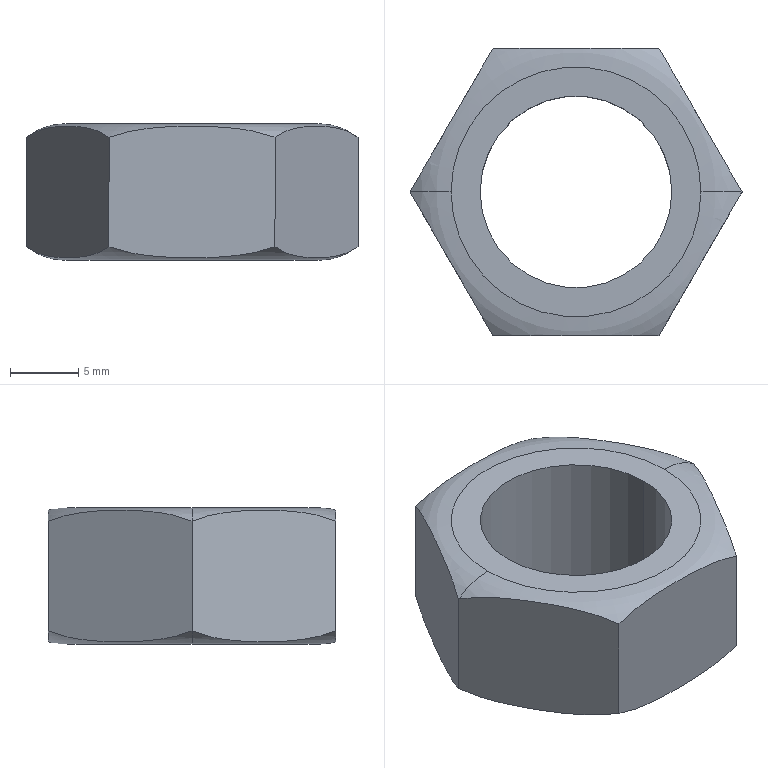Part | SolidWorks | features Extrusion 1, ICE 1, RevCut 1 | 1 solid | 14 faces | box 24.249 x 21 x 10 mm | volume 2242 mm3 | plane 8 | torus 4 | cylinder 2 | commonest cylinder face diameters 14 x2
STEP:
#1=CARTESIAN_POINT('',(7.,0.,10.));
#2=VERTEX_POINT('',#1);
#3=CARTESIAN_POINT('',(-7.,0.,10.));
#4=VERTEX_POINT('',#3);
#5=CARTESIAN_POINT('',(0.,0.,10.));
#6=DIRECTION('',(0.,0.,-1.));
#7=DIRECTION('',(-1.,0.,0.));
#8=AXIS2_PLACEMENT_3D('',#5,#6,#7);
#9=CIRCLE('',#8,7.);
#10=EDGE_CURVE('',#2,#4,#9,.T.);
#11=ORIENTED_EDGE('',*,*,#10,.F.);
#12=CARTESIAN_POINT('',(7.,0.,0.));
#13=VERTEX_POINT('',#12);
#14=CARTESIAN_POINT('',(7.,0.,10.));
#15=DIRECTION('',(0.,0.,-1.));
#16=VECTOR('',#15,1000.);
#17=LINE('',#14,#16);
#18=EDGE_CURVE('',#2,#13,#17,.T.);
#19=ORIENTED_EDGE('',*,*,#18,.T.);
#20=CARTESIAN_POINT('',(-7.,0.,0.));
#21=VERTEX_POINT('',#20);
#22=CARTESIAN_POINT('',(0.,0.,0.));
#23=DIRECTION('',(0.,0.,-1.));
#24=DIRECTION('',(-1.,0.,0.));
#25=AXIS2_PLACEMENT_3D('',#22,#23,#24);
#26=CIRCLE('',#25,7.);
#27=EDGE_CURVE('',#13,#21,#26,.T.);
#28=ORIENTED_EDGE('',*,*,#27,.T.);
#29=CARTESIAN_POINT('',(-7.,0.,10.));
#30=DIRECTION('',(0.,0.,-1.));
#31=VECTOR('',#30,1000.);
#32=LINE('',#29,#31);
#33=EDGE_CURVE('',#4,#21,#32,.T.);
#34=ORIENTED_EDGE('',*,*,#33,.F.);
#35=EDGE_LOOP('',(#11,#19,#28,#34));
#36=FACE_OUTER_BOUND('',#35,.T.);
#37=CARTESIAN_POINT('',(0.,0.,10.));
#38=DIRECTION('',(0.,0.,-1.));
#39=DIRECTION('',(-1.,0.,0.));
#40=AXIS2_PLACEMENT_3D('',#37,#38,#39);
#41=CYLINDRICAL_SURFACE('',#40,7.);
#42=ADVANCED_FACE('',(#36),#41,.F.);
#43=CARTESIAN_POINT('',(-9.124,0.,10.));
#44=VERTEX_POINT('',#43);
#45=CARTESIAN_POINT('',(9.124,0.,10.));
#46=VERTEX_POINT('',#45);
#47=CARTESIAN_POINT('',(0.,0.,10.));
#48=DIRECTION('',(0.,0.,-1.));
#49=DIRECTION('',(-1.,0.,0.));
#50=AXIS2_PLACEMENT_3D('',#47,#48,#49);
#51=CIRCLE('',#50,9.124);
#52=EDGE_CURVE('',#44,#46,#51,.T.);
#53=ORIENTED_EDGE('',*,*,#52,.T.);
#54=CARTESIAN_POINT('',(12.124,0.,9.));
#55=VERTEX_POINT('',#54);
#56=CARTESIAN_POINT('',(9.124,0.,5.));
#57=DIRECTION('',(0.,1.,0.));
#58=DIRECTION('',(-1.,0.,0.));
#59=AXIS2_PLACEMENT_3D('',#56,#57,#58);
#60=CIRCLE('',#59,5.);
#61=EDGE_CURVE('',#46,#55,#60,.T.);
#62=ORIENTED_EDGE('',*,*,#61,.T.);
#63=CARTESIAN_POINT('',(6.062,10.5,9.));
#64=VERTEX_POINT('',#63);
#65=CARTESIAN_POINT('',(6.062,10.5,9.));
#66=CARTESIAN_POINT('',(6.304,10.08,9.182));
#67=CARTESIAN_POINT('',(6.551,9.653,9.317));
#68=CARTESIAN_POINT('',(7.05,8.789,9.528));
#69=CARTESIAN_POINT('',(7.303,8.351,9.603));
#70=CARTESIAN_POINT('',(7.811,7.47,9.714));
#71=CARTESIAN_POINT('',(8.068,7.026,9.75));
#72=CARTESIAN_POINT('',(8.58,6.139,9.797));
#73=CARTESIAN_POINT('',(8.835,5.696,9.807));
#74=CARTESIAN_POINT('',(9.346,4.812,9.807));
#75=CARTESIAN_POINT('',(9.602,4.37,9.797));
#76=CARTESIAN_POINT('',(10.112,3.486,9.751));
#77=CARTESIAN_POINT('',(10.366,3.045,9.716));
#78=CARTESIAN_POINT('',(10.875,2.164,9.605));
#79=CARTESIAN_POINT('',(11.13,1.722,9.53));
#80=CARTESIAN_POINT('',(11.634,0.8487,9.318));
#81=CARTESIAN_POINT('',(11.882,0.419,9.181));
#82=CARTESIAN_POINT('',(12.124,0.,9.));
#83=B_SPLINE_CURVE_WITH_KNOTS('',3,(#65,#66,#67,#68,#69,#70,#71,#72,#73,#74,#75,#76,#77,#78,#79,#80,#81,#82),.UNSPECIFIED.,.F.,.F.,(4,2,2,2,2,2,2,2,4),(0.000000243,0.00153,0.003061,0.004591,0.006121,0.007651,0.009181,0.01071,0.01224),.UNSPECIFIED.);
#84=EDGE_CURVE('',#64,#55,#83,.T.);
#85=ORIENTED_EDGE('',*,*,#84,.F.);
#86=CARTESIAN_POINT('',(-6.062,10.5,9.));
#87=VERTEX_POINT('',#86);
#88=CARTESIAN_POINT('',(-6.062,10.5,9.));
#89=CARTESIAN_POINT('',(-5.582,10.5,9.18));
#90=CARTESIAN_POINT('',(-5.091,10.5,9.315));
#91=CARTESIAN_POINT('',(-4.093,10.5,9.526));
#92=CARTESIAN_POINT('',(-3.587,10.5,9.602));
#93=CARTESIAN_POINT('',(-2.567,10.5,9.714));
#94=CARTESIAN_POINT('',(-2.056,10.5,9.75));
#95=CARTESIAN_POINT('',(-1.033,10.5,9.796));
#96=CARTESIAN_POINT('',(-0.5206,10.5,9.807));
#97=CARTESIAN_POINT('',(0.5051,10.5,9.807));
#98=CARTESIAN_POINT('',(1.018,10.5,9.797));
#99=CARTESIAN_POINT('',(2.041,10.5,9.751));
#100=CARTESIAN_POINT('',(2.551,10.5,9.715));
#101=CARTESIAN_POINT('',(3.568,10.5,9.605));
#102=CARTESIAN_POINT('',(4.074,10.5,9.53));
#103=CARTESIAN_POINT('',(5.081,10.5,9.318));
#104=CARTESIAN_POINT('',(5.581,10.5,9.181));
#105=CARTESIAN_POINT('',(6.062,10.5,9.));
#106=B_SPLINE_CURVE_WITH_KNOTS('',3,(#88,#89,#90,#91,#92,#93,#94,#95,#96,#97,#98,#99,#100,#101,#102,#103,#104,#105),.UNSPECIFIED.,.F.,.F.,(4,2,2,2,2,2,2,2,4),(0.04063,0.04216,0.0437,0.04523,0.04676,0.0483,0.04983,0.05136,0.0529),.UNSPECIFIED.);
#107=EDGE_CURVE('',#87,#64,#106,.T.);
#108=ORIENTED_EDGE('',*,*,#107,.F.);
#109=CARTESIAN_POINT('',(-12.124,0.,9.));
#110=VERTEX_POINT('',#109);
#111=CARTESIAN_POINT('',(-12.124,0.,9.));
#112=CARTESIAN_POINT('',(-11.882,0.4195,9.182));
#113=CARTESIAN_POINT('',(-11.635,0.8468,9.317));
#114=CARTESIAN_POINT('',(-11.136,1.711,9.528));
#115=CARTESIAN_POINT('',(-10.884,2.149,9.603));
#116=CARTESIAN_POINT('',(-10.375,3.03,9.714));
#117=CARTESIAN_POINT('',(-10.118,3.474,9.75));
#118=CARTESIAN_POINT('',(-9.607,4.361,9.797));
#119=CARTESIAN_POINT('',(-9.351,4.804,9.807));
#120=CARTESIAN_POINT('',(-8.84,5.688,9.807));
#121=CARTESIAN_POINT('',(-8.585,6.13,9.797));
#122=CARTESIAN_POINT('',(-8.075,7.014,9.751));
#123=CARTESIAN_POINT('',(-7.82,7.455,9.716));
#124=CARTESIAN_POINT('',(-7.311,8.336,9.605));
#125=CARTESIAN_POINT('',(-7.056,8.778,9.53));
#126=CARTESIAN_POINT('',(-6.552,9.651,9.318));
#127=CARTESIAN_POINT('',(-6.304,10.081,9.181));
#128=CARTESIAN_POINT('',(-6.062,10.5,9.));
#129=B_SPLINE_CURVE_WITH_KNOTS('',3,(#111,#112,#113,#114,#115,#116,#117,#118,#119,#120,#121,#122,#123,#124,#125,#126,#127,#128),.UNSPECIFIED.,.F.,.F.,(4,2,2,2,2,2,2,2,4),(0.000000243,0.00153,0.003061,0.004591,0.006121,0.007651,0.009181,0.01071,0.01224),.UNSPECIFIED.);
#130=EDGE_CURVE('',#110,#87,#129,.T.);
#131=ORIENTED_EDGE('',*,*,#130,.F.);
#132=CARTESIAN_POINT('',(-9.124,0.,5.));
#133=DIRECTION('',(0.,-1.,0.));
#134=DIRECTION('',(0.,0.,-1.));
#135=AXIS2_PLACEMENT_3D('',#132,#133,#134);
#136=CIRCLE('',#135,5.);
#137=EDGE_CURVE('',#44,#110,#136,.T.);
#138=ORIENTED_EDGE('',*,*,#137,.F.);
#139=EDGE_LOOP('',(#53,#62,#85,#108,#131,#138));
#140=FACE_OUTER_BOUND('',#139,.T.);
#141=CARTESIAN_POINT('',(0.,0.,5.));
#142=DIRECTION('',(0.,0.,-1.));
#143=DIRECTION('',(-1.,0.,0.));
#144=AXIS2_PLACEMENT_3D('',#141,#142,#143);
#145=TOROIDAL_SURFACE('',#144,9.124,5.);
#146=ADVANCED_FACE('',(#140),#145,.T.);
#147=CARTESIAN_POINT('',(12.124,0.,1.));
#148=VERTEX_POINT('',#147);
#149=CARTESIAN_POINT('',(6.062,10.5,1.));
#150=VERTEX_POINT('',#149);
#151=CARTESIAN_POINT('',(12.124,0.,1.));
#152=CARTESIAN_POINT('',(11.882,0.4195,0.8183));
#153=CARTESIAN_POINT('',(11.635,0.8468,0.6831));
#154=CARTESIAN_POINT('',(11.136,1.711,0.4723));
#155=CARTESIAN_POINT('',(10.884,2.149,0.3971));
#156=CARTESIAN_POINT('',(10.375,3.03,0.2857));
#157=CARTESIAN_POINT('',(10.118,3.474,0.2496));
#158=CARTESIAN_POINT('',(9.607,4.361,0.2034));
#159=CARTESIAN_POINT('',(9.351,4.804,0.193));
#160=CARTESIAN_POINT('',(8.84,5.688,0.1929));
#161=CARTESIAN_POINT('',(8.585,6.13,0.2031));
#162=CARTESIAN_POINT('',(8.075,7.014,0.2488));
#163=CARTESIAN_POINT('',(7.82,7.455,0.2843));
#164=CARTESIAN_POINT('',(7.311,8.336,0.3947));
#165=CARTESIAN_POINT('',(7.056,8.778,0.47));
#166=CARTESIAN_POINT('',(6.552,9.651,0.6823));
#167=CARTESIAN_POINT('',(6.304,10.081,0.8186));
#168=CARTESIAN_POINT('',(6.062,10.5,1.));
#169=B_SPLINE_CURVE_WITH_KNOTS('',3,(#151,#152,#153,#154,#155,#156,#157,#158,#159,#160,#161,#162,#163,#164,#165,#166,#167,#168),.UNSPECIFIED.,.F.,.F.,(4,2,2,2,2,2,2,2,4),(0.000000243,0.00153,0.003061,0.004591,0.006121,0.007651,0.009181,0.01071,0.01224),.UNSPECIFIED.);
#170=EDGE_CURVE('',#148,#150,#169,.T.);
#171=ORIENTED_EDGE('',*,*,#170,.F.);
#172=CARTESIAN_POINT('',(9.124,0.,0.));
#173=VERTEX_POINT('',#172);
#174=CARTESIAN_POINT('',(9.124,0.,5.));
#175=DIRECTION('',(0.,1.,0.));
#176=DIRECTION('',(-1.,0.,0.));
#177=AXIS2_PLACEMENT_3D('',#174,#175,#176);
#178=CIRCLE('',#177,5.);
#179=EDGE_CURVE('',#148,#173,#178,.T.);
#180=ORIENTED_EDGE('',*,*,#179,.T.);
#181=CARTESIAN_POINT('',(-9.124,0.,0.));
#182=VERTEX_POINT('',#181);
#183=CARTESIAN_POINT('',(0.,0.,0.));
#184=DIRECTION('',(0.,0.,-1.));
#185=DIRECTION('',(-1.,0.,0.));
#186=AXIS2_PLACEMENT_3D('',#183,#184,#185);
#187=CIRCLE('',#186,9.124);
#188=EDGE_CURVE('',#182,#173,#187,.T.);
#189=ORIENTED_EDGE('',*,*,#188,.F.);
#190=CARTESIAN_POINT('',(-12.124,0.,1.));
#191=VERTEX_POINT('',#190);
#192=CARTESIAN_POINT('',(-9.124,0.,5.));
#193=DIRECTION('',(0.,-1.,0.));
#194=DIRECTION('',(0.,0.,-1.));
#195=AXIS2_PLACEMENT_3D('',#192,#193,#194);
#196=CIRCLE('',#195,5.);
#197=EDGE_CURVE('',#191,#182,#196,.T.);
#198=ORIENTED_EDGE('',*,*,#197,.F.);
#199=CARTESIAN_POINT('',(-6.062,10.5,1.));
#200=VERTEX_POINT('',#199);
#201=CARTESIAN_POINT('',(-6.062,10.5,1.));
#202=CARTESIAN_POINT('',(-6.304,10.08,0.8183));
#203=CARTESIAN_POINT('',(-6.551,9.653,0.6831));
#204=CARTESIAN_POINT('',(-7.05,8.789,0.4723));
#205=CARTESIAN_POINT('',(-7.303,8.351,0.3971));
#206=CARTESIAN_POINT('',(-7.811,7.47,0.2857));
#207=CARTESIAN_POINT('',(-8.068,7.026,0.2496));
#208=CARTESIAN_POINT('',(-8.58,6.139,0.2034));
#209=CARTESIAN_POINT('',(-8.835,5.696,0.193));
#210=CARTESIAN_POINT('',(-9.346,4.812,0.1929));
#211=CARTESIAN_POINT('',(-9.602,4.37,0.2031));
#212=CARTESIAN_POINT('',(-10.112,3.486,0.2488));
#213=CARTESIAN_POINT('',(-10.366,3.045,0.2843));
#214=CARTESIAN_POINT('',(-10.875,2.164,0.3947));
#215=CARTESIAN_POINT('',(-11.13,1.722,0.47));
#216=CARTESIAN_POINT('',(-11.634,0.8487,0.6823));
#217=CARTESIAN_POINT('',(-11.882,0.419,0.8186));
#218=CARTESIAN_POINT('',(-12.124,0.,1.));
#219=B_SPLINE_CURVE_WITH_KNOTS('',3,(#201,#202,#203,#204,#205,#206,#207,#208,#209,#210,#211,#212,#213,#214,#215,#216,#217,#218),.UNSPECIFIED.,.F.,.F.,(4,2,2,2,2,2,2,2,4),(0.000000243,0.00153,0.003061,0.004591,0.006121,0.007651,0.009181,0.01071,0.01224),.UNSPECIFIED.);
#220=EDGE_CURVE('',#200,#191,#219,.T.);
#221=ORIENTED_EDGE('',*,*,#220,.F.);
#222=CARTESIAN_POINT('',(6.062,10.5,1.));
#223=CARTESIAN_POINT('',(5.582,10.5,0.8199));
#224=CARTESIAN_POINT('',(5.091,10.5,0.6847));
#225=CARTESIAN_POINT('',(4.093,10.5,0.4736));
#226=CARTESIAN_POINT('',(3.587,10.5,0.3979));
#227=CARTESIAN_POINT('',(2.567,10.5,0.286));
#228=CARTESIAN_POINT('',(2.056,10.5,0.25));
#229=CARTESIAN_POINT('',(1.033,10.5,0.2035));
#230=CARTESIAN_POINT('',(0.5206,10.5,0.1931));
#231=CARTESIAN_POINT('',(-0.5051,10.5,0.1929));
#232=CARTESIAN_POINT('',(-1.018,10.5,0.2031));
#233=CARTESIAN_POINT('',(-2.041,10.5,0.249));
#234=CARTESIAN_POINT('',(-2.551,10.5,0.2847));
#235=CARTESIAN_POINT('',(-3.568,10.5,0.3953));
#236=CARTESIAN_POINT('',(-4.074,10.5,0.4702));
#237=CARTESIAN_POINT('',(-5.081,10.5,0.6821));
#238=CARTESIAN_POINT('',(-5.581,10.5,0.8195));
#239=CARTESIAN_POINT('',(-6.062,10.5,1.));
#240=B_SPLINE_CURVE_WITH_KNOTS('',3,(#222,#223,#224,#225,#226,#227,#228,#229,#230,#231,#232,#233,#234,#235,#236,#237,#238,#239),.UNSPECIFIED.,.F.,.F.,(4,2,2,2,2,2,2,2,4),(0.04063,0.04216,0.0437,0.04523,0.04676,0.0483,0.04983,0.05136,0.0529),.UNSPECIFIED.);
#241=EDGE_CURVE('',#150,#200,#240,.T.);
#242=ORIENTED_EDGE('',*,*,#241,.F.);
#243=EDGE_LOOP('',(#171,#180,#189,#198,#221,#242));
#244=FACE_OUTER_BOUND('',#243,.T.);
#245=CARTESIAN_POINT('',(0.,0.,5.));
#246=DIRECTION('',(0.,0.,-1.));
#247=DIRECTION('',(-1.,0.,0.));
#248=AXIS2_PLACEMENT_3D('',#245,#246,#247);
#249=TOROIDAL_SURFACE('',#248,9.124,5.);
#250=ADVANCED_FACE('',(#244),#249,.T.);
#251=CARTESIAN_POINT('',(12.124,0.,10.));
#252=DIRECTION('',(0.,0.,-1.));
#253=VECTOR('',#252,1000.);
#254=LINE('',#251,#253);
#255=EDGE_CURVE('',#55,#148,#254,.T.);
#256=ORIENTED_EDGE('',*,*,#255,.F.);
#257=CARTESIAN_POINT('',(6.062,-10.5,9.));
#258=VERTEX_POINT('',#257);
#259=CARTESIAN_POINT('',(12.124,0.,9.));
#260=CARTESIAN_POINT('',(11.882,-0.4195,9.182));
#261=CARTESIAN_POINT('',(11.635,-0.8468,9.317));
#262=CARTESIAN_POINT('',(11.136,-1.711,9.528));
#263=CARTESIAN_POINT('',(10.884,-2.149,9.603));
#264=CARTESIAN_POINT('',(10.375,-3.03,9.714));
#265=CARTESIAN_POINT('',(10.118,-3.474,9.75));
#266=CARTESIAN_POINT('',(9.607,-4.361,9.797));
#267=CARTESIAN_POINT('',(9.351,-4.804,9.807));
#268=CARTESIAN_POINT('',(8.84,-5.688,9.807));
#269=CARTESIAN_POINT('',(8.585,-6.13,9.797));
#270=CARTESIAN_POINT('',(8.075,-7.014,9.751));
#271=CARTESIAN_POINT('',(7.82,-7.455,9.716));
#272=CARTESIAN_POINT('',(7.311,-8.336,9.605));
#273=CARTESIAN_POINT('',(7.056,-8.778,9.53));
#274=CARTESIAN_POINT('',(6.552,-9.651,9.318));
#275=CARTESIAN_POINT('',(6.304,-10.081,9.181));
#276=CARTESIAN_POINT('',(6.062,-10.5,9.));
#277=B_SPLINE_CURVE_WITH_KNOTS('',3,(#259,#260,#261,#262,#263,#264,#265,#266,#267,#268,#269,#270,#271,#272,#273,#274,#275,#276),.UNSPECIFIED.,.F.,.F.,(4,2,2,2,2,2,2,2,4),(0.000000243,0.00153,0.003061,0.004591,0.006121,0.007651,0.009181,0.01071,0.01224),.UNSPECIFIED.);
#278=EDGE_CURVE('',#55,#258,#277,.T.);
#279=ORIENTED_EDGE('',*,*,#278,.T.);
#280=CARTESIAN_POINT('',(6.062,-10.5,1.));
#281=VERTEX_POINT('',#280);
#282=CARTESIAN_POINT('',(6.062,-10.5,10.));
#283=DIRECTION('',(0.,0.,-1.));
#284=VECTOR('',#283,1000.);
#285=LINE('',#282,#284);
#286=EDGE_CURVE('',#258,#281,#285,.T.);
#287=ORIENTED_EDGE('',*,*,#286,.T.);
#288=CARTESIAN_POINT('',(6.062,-10.5,1.));
#289=CARTESIAN_POINT('',(6.304,-10.08,0.8183));
#290=CARTESIAN_POINT('',(6.551,-9.653,0.6831));
#291=CARTESIAN_POINT('',(7.05,-8.789,0.4723));
#292=CARTESIAN_POINT('',(7.303,-8.351,0.3971));
#293=CARTESIAN_POINT('',(7.811,-7.47,0.2857));
#294=CARTESIAN_POINT('',(8.068,-7.026,0.2496));
#295=CARTESIAN_POINT('',(8.58,-6.139,0.2034));
#296=CARTESIAN_POINT('',(8.835,-5.696,0.193));
#297=CARTESIAN_POINT('',(9.346,-4.812,0.1929));
#298=CARTESIAN_POINT('',(9.602,-4.37,0.2031));
#299=CARTESIAN_POINT('',(10.112,-3.486,0.2488));
#300=CARTESIAN_POINT('',(10.366,-3.045,0.2843));
#301=CARTESIAN_POINT('',(10.875,-2.164,0.3947));
#302=CARTESIAN_POINT('',(11.13,-1.722,0.47));
#303=CARTESIAN_POINT('',(11.634,-0.8487,0.6823));
#304=CARTESIAN_POINT('',(11.882,-0.419,0.8186));
#305=CARTESIAN_POINT('',(12.124,0.,1.));
#306=B_SPLINE_CURVE_WITH_KNOTS('',3,(#288,#289,#290,#291,#292,#293,#294,#295,#296,#297,#298,#299,#300,#301,#302,#303,#304,#305),.UNSPECIFIED.,.F.,.F.,(4,2,2,2,2,2,2,2,4),(0.000000243,0.00153,0.003061,0.004591,0.006121,0.007651,0.009181,0.01071,0.01224),.UNSPECIFIED.);
#307=EDGE_CURVE('',#281,#148,#306,.T.);
#308=ORIENTED_EDGE('',*,*,#307,.T.);
#309=EDGE_LOOP('',(#256,#279,#287,#308));
#310=FACE_OUTER_BOUND('',#309,.T.);
#311=CARTESIAN_POINT('',(6.062,-10.5,10.));
#312=DIRECTION('',(-0.866,0.5,0.));
#313=DIRECTION('',(-0.5,-0.866,0.));
#314=AXIS2_PLACEMENT_3D('',#311,#312,#313);
#315=PLANE('',#314);
#316=ADVANCED_FACE('',(#310),#315,.F.);
#317=CARTESIAN_POINT('',(6.062,10.5,10.));
#318=DIRECTION('',(0.,0.,-1.));
#319=VECTOR('',#318,1000.);
#320=LINE('',#317,#319);
#321=EDGE_CURVE('',#64,#150,#320,.T.);
#322=ORIENTED_EDGE('',*,*,#321,.F.);
#323=ORIENTED_EDGE('',*,*,#84,.T.);
#324=ORIENTED_EDGE('',*,*,#255,.T.);
#325=ORIENTED_EDGE('',*,*,#170,.T.);
#326=EDGE_LOOP('',(#322,#323,#324,#325));
#327=FACE_OUTER_BOUND('',#326,.T.);
#328=CARTESIAN_POINT('',(12.124,0.,10.));
#329=DIRECTION('',(-0.866,-0.5,0.));
#330=DIRECTION('',(0.5,-0.866,0.));
#331=AXIS2_PLACEMENT_3D('',#328,#329,#330);
#332=PLANE('',#331);
#333=ADVANCED_FACE('',(#327),#332,.F.);
#334=CARTESIAN_POINT('',(-6.062,10.5,10.));
#335=DIRECTION('',(0.,0.,-1.));
#336=VECTOR('',#335,1000.);
#337=LINE('',#334,#336);
#338=EDGE_CURVE('',#87,#200,#337,.T.);
#339=ORIENTED_EDGE('',*,*,#338,.F.);
#340=ORIENTED_EDGE('',*,*,#107,.T.);
#341=ORIENTED_EDGE('',*,*,#321,.T.);
#342=ORIENTED_EDGE('',*,*,#241,.T.);
#343=EDGE_LOOP('',(#339,#340,#341,#342));
#344=FACE_OUTER_BOUND('',#343,.T.);
#345=CARTESIAN_POINT('',(6.062,10.5,10.));
#346=DIRECTION('',(0.,-1.,0.));
#347=DIRECTION('',(0.,0.,-1.));
#348=AXIS2_PLACEMENT_3D('',#345,#346,#347);
#349=PLANE('',#348);
#350=ADVANCED_FACE('',(#344),#349,.F.);
#351=CARTESIAN_POINT('',(-12.124,0.,10.));
#352=DIRECTION('',(0.,0.,-1.));
#353=VECTOR('',#352,1000.);
#354=LINE('',#351,#353);
#355=EDGE_CURVE('',#110,#191,#354,.T.);
#356=ORIENTED_EDGE('',*,*,#355,.F.);
#357=ORIENTED_EDGE('',*,*,#130,.T.);
#358=ORIENTED_EDGE('',*,*,#338,.T.);
#359=ORIENTED_EDGE('',*,*,#220,.T.);
#360=EDGE_LOOP('',(#356,#357,#358,#359));
#361=FACE_OUTER_BOUND('',#360,.T.);
#362=CARTESIAN_POINT('',(-6.062,10.5,10.));
#363=DIRECTION('',(0.866,-0.5,0.));
#364=DIRECTION('',(0.5,0.866,0.));
#365=AXIS2_PLACEMENT_3D('',#362,#363,#364);
#366=PLANE('',#365);
#367=ADVANCED_FACE('',(#361),#366,.F.);
#368=CARTESIAN_POINT('',(-6.062,-10.5,9.));
#369=VERTEX_POINT('',#368);
#370=CARTESIAN_POINT('',(-6.062,-10.5,1.));
#371=VERTEX_POINT('',#370);
#372=CARTESIAN_POINT('',(-6.062,-10.5,10.));
#373=DIRECTION('',(0.,0.,-1.));
#374=VECTOR('',#373,1000.);
#375=LINE('',#372,#374);
#376=EDGE_CURVE('',#369,#371,#375,.T.);
#377=ORIENTED_EDGE('',*,*,#376,.F.);
#378=CARTESIAN_POINT('',(-6.062,-10.5,9.));
#379=CARTESIAN_POINT('',(-6.304,-10.08,9.182));
#380=CARTESIAN_POINT('',(-6.551,-9.653,9.317));
#381=CARTESIAN_POINT('',(-7.05,-8.789,9.528));
#382=CARTESIAN_POINT('',(-7.303,-8.351,9.603));
#383=CARTESIAN_POINT('',(-7.811,-7.47,9.714));
#384=CARTESIAN_POINT('',(-8.068,-7.026,9.75));
#385=CARTESIAN_POINT('',(-8.58,-6.139,9.797));
#386=CARTESIAN_POINT('',(-8.835,-5.696,9.807));
#387=CARTESIAN_POINT('',(-9.346,-4.812,9.807));
#388=CARTESIAN_POINT('',(-9.602,-4.37,9.797));
#389=CARTESIAN_POINT('',(-10.112,-3.486,9.751));
#390=CARTESIAN_POINT('',(-10.366,-3.045,9.716));
#391=CARTESIAN_POINT('',(-10.875,-2.164,9.605));
#392=CARTESIAN_POINT('',(-11.13,-1.722,9.53));
#393=CARTESIAN_POINT('',(-11.634,-0.8487,9.318));
#394=CARTESIAN_POINT('',(-11.882,-0.419,9.181));
#395=CARTESIAN_POINT('',(-12.124,0.,9.));
#396=B_SPLINE_CURVE_WITH_KNOTS('',3,(#378,#379,#380,#381,#382,#383,#384,#385,#386,#387,#388,#389,#390,#391,#392,#393,#394,#395),.UNSPECIFIED.,.F.,.F.,(4,2,2,2,2,2,2,2,4),(0.000000243,0.00153,0.003061,0.004591,0.006121,0.007651,0.009181,0.01071,0.01224),.UNSPECIFIED.);
#397=EDGE_CURVE('',#369,#110,#396,.T.);
#398=ORIENTED_EDGE('',*,*,#397,.T.);
#399=ORIENTED_EDGE('',*,*,#355,.T.);
#400=CARTESIAN_POINT('',(-12.124,0.,1.));
#401=CARTESIAN_POINT('',(-11.882,-0.4195,0.8183));
#402=CARTESIAN_POINT('',(-11.635,-0.8468,0.6831));
#403=CARTESIAN_POINT('',(-11.136,-1.711,0.4723));
#404=CARTESIAN_POINT('',(-10.884,-2.149,0.3971));
#405=CARTESIAN_POINT('',(-10.375,-3.03,0.2857));
#406=CARTESIAN_POINT('',(-10.118,-3.474,0.2496));
#407=CARTESIAN_POINT('',(-9.607,-4.361,0.2034));
#408=CARTESIAN_POINT('',(-9.351,-4.804,0.193));
#409=CARTESIAN_POINT('',(-8.84,-5.688,0.1929));
#410=CARTESIAN_POINT('',(-8.585,-6.13,0.2031));
#411=CARTESIAN_POINT('',(-8.075,-7.014,0.2488));
#412=CARTESIAN_POINT('',(-7.82,-7.455,0.2843));
#413=CARTESIAN_POINT('',(-7.311,-8.336,0.3947));
#414=CARTESIAN_POINT('',(-7.056,-8.778,0.47));
#415=CARTESIAN_POINT('',(-6.552,-9.651,0.6823));
#416=CARTESIAN_POINT('',(-6.304,-10.081,0.8186));
#417=CARTESIAN_POINT('',(-6.062,-10.5,1.));
#418=B_SPLINE_CURVE_WITH_KNOTS('',3,(#400,#401,#402,#403,#404,#405,#406,#407,#408,#409,#410,#411,#412,#413,#414,#415,#416,#417),.UNSPECIFIED.,.F.,.F.,(4,2,2,2,2,2,2,2,4),(0.000000243,0.00153,0.003061,0.004591,0.006121,0.007651,0.009181,0.01071,0.01224),.UNSPECIFIED.);
#419=EDGE_CURVE('',#191,#371,#418,.T.);
#420=ORIENTED_EDGE('',*,*,#419,.T.);
#421=EDGE_LOOP('',(#377,#398,#399,#420));
#422=FACE_OUTER_BOUND('',#421,.T.);
#423=CARTESIAN_POINT('',(-12.124,0.,10.));
#424=DIRECTION('',(0.866,0.5,0.));
#425=DIRECTION('',(-0.5,0.866,0.));
#426=AXIS2_PLACEMENT_3D('',#423,#424,#425);
#427=PLANE('',#426);
#428=ADVANCED_FACE('',(#422),#427,.F.);
#429=ORIENTED_EDGE('',*,*,#286,.F.);
#430=CARTESIAN_POINT('',(6.062,-10.5,9.));
#431=CARTESIAN_POINT('',(5.582,-10.5,9.18));
#432=CARTESIAN_POINT('',(5.091,-10.5,9.315));
#433=CARTESIAN_POINT('',(4.093,-10.5,9.526));
#434=CARTESIAN_POINT('',(3.587,-10.5,9.602));
#435=CARTESIAN_POINT('',(2.567,-10.5,9.714));
#436=CARTESIAN_POINT('',(2.056,-10.5,9.75));
#437=CARTESIAN_POINT('',(1.033,-10.5,9.796));
#438=CARTESIAN_POINT('',(0.5206,-10.5,9.807));
#439=CARTESIAN_POINT('',(-0.5051,-10.5,9.807));
#440=CARTESIAN_POINT('',(-1.018,-10.5,9.797));
#441=CARTESIAN_POINT('',(-2.041,-10.5,9.751));
#442=CARTESIAN_POINT('',(-2.551,-10.5,9.715));
#443=CARTESIAN_POINT('',(-3.568,-10.5,9.605));
#444=CARTESIAN_POINT('',(-4.074,-10.5,9.53));
#445=CARTESIAN_POINT('',(-5.081,-10.5,9.318));
#446=CARTESIAN_POINT('',(-5.581,-10.5,9.181));
#447=CARTESIAN_POINT('',(-6.062,-10.5,9.));
#448=B_SPLINE_CURVE_WITH_KNOTS('',3,(#430,#431,#432,#433,#434,#435,#436,#437,#438,#439,#440,#441,#442,#443,#444,#445,#446,#447),.UNSPECIFIED.,.F.,.F.,(4,2,2,2,2,2,2,2,4),(0.04063,0.04216,0.0437,0.04523,0.04676,0.0483,0.04983,0.05136,0.0529),.UNSPECIFIED.);
#449=EDGE_CURVE('',#258,#369,#448,.T.);
#450=ORIENTED_EDGE('',*,*,#449,.T.);
#451=ORIENTED_EDGE('',*,*,#376,.T.);
#452=CARTESIAN_POINT('',(-6.062,-10.5,1.));
#453=CARTESIAN_POINT('',(-5.582,-10.5,0.8199));
#454=CARTESIAN_POINT('',(-5.091,-10.5,0.6847));
#455=CARTESIAN_POINT('',(-4.093,-10.5,0.4736));
#456=CARTESIAN_POINT('',(-3.587,-10.5,0.3979));
#457=CARTESIAN_POINT('',(-2.567,-10.5,0.286));
#458=CARTESIAN_POINT('',(-2.056,-10.5,0.25));
#459=CARTESIAN_POINT('',(-1.033,-10.5,0.2035));
#460=CARTESIAN_POINT('',(-0.5206,-10.5,0.1931));
#461=CARTESIAN_POINT('',(0.5051,-10.5,0.1929));
#462=CARTESIAN_POINT('',(1.018,-10.5,0.2031));
#463=CARTESIAN_POINT('',(2.041,-10.5,0.249));
#464=CARTESIAN_POINT('',(2.551,-10.5,0.2847));
#465=CARTESIAN_POINT('',(3.568,-10.5,0.3953));
#466=CARTESIAN_POINT('',(4.074,-10.5,0.4702));
#467=CARTESIAN_POINT('',(5.081,-10.5,0.6821));
#468=CARTESIAN_POINT('',(5.581,-10.5,0.8195));
#469=CARTESIAN_POINT('',(6.062,-10.5,1.));
#470=B_SPLINE_CURVE_WITH_KNOTS('',3,(#452,#453,#454,#455,#456,#457,#458,#459,#460,#461,#462,#463,#464,#465,#466,#467,#468,#469),.UNSPECIFIED.,.F.,.F.,(4,2,2,2,2,2,2,2,4),(0.04063,0.04216,0.0437,0.04523,0.04676,0.0483,0.04983,0.05136,0.0529),.UNSPECIFIED.);
#471=EDGE_CURVE('',#371,#281,#470,.T.);
#472=ORIENTED_EDGE('',*,*,#471,.T.);
#473=EDGE_LOOP('',(#429,#450,#451,#472));
#474=FACE_OUTER_BOUND('',#473,.T.);
#475=CARTESIAN_POINT('',(-6.062,-10.5,10.));
#476=DIRECTION('',(0.,1.,0.));
#477=DIRECTION('',(0.,0.,1.));
#478=AXIS2_PLACEMENT_3D('',#475,#476,#477);
#479=PLANE('',#478);
#480=ADVANCED_FACE('',(#474),#479,.F.);
#481=ORIENTED_EDGE('',*,*,#179,.F.);
#482=ORIENTED_EDGE('',*,*,#307,.F.);
#483=ORIENTED_EDGE('',*,*,#471,.F.);
#484=ORIENTED_EDGE('',*,*,#419,.F.);
#485=ORIENTED_EDGE('',*,*,#197,.T.);
#486=CARTESIAN_POINT('',(0.,0.,0.));
#487=DIRECTION('',(0.,0.,-1.));
#488=DIRECTION('',(-1.,0.,0.));
#489=AXIS2_PLACEMENT_3D('',#486,#487,#488);
#490=CIRCLE('',#489,9.124);
#491=EDGE_CURVE('',#173,#182,#490,.T.);
#492=ORIENTED_EDGE('',*,*,#491,.F.);
#493=EDGE_LOOP('',(#481,#482,#483,#484,#485,#492));
#494=FACE_OUTER_BOUND('',#493,.T.);
#495=CARTESIAN_POINT('',(0.,0.,5.));
#496=DIRECTION('',(0.,0.,-1.));
#497=DIRECTION('',(-1.,0.,0.));
#498=AXIS2_PLACEMENT_3D('',#495,#496,#497);
#499=TOROIDAL_SURFACE('',#498,9.124,5.);
#500=ADVANCED_FACE('',(#494),#499,.T.);
#501=CARTESIAN_POINT('',(0.,0.,0.));
#502=DIRECTION('',(0.,0.,-1.));
#503=DIRECTION('',(-1.,0.,0.));
#504=AXIS2_PLACEMENT_3D('',#501,#502,#503);
#505=CIRCLE('',#504,7.);
#506=EDGE_CURVE('',#21,#13,#505,.T.);
#507=ORIENTED_EDGE('',*,*,#506,.F.);
#508=ORIENTED_EDGE('',*,*,#27,.F.);
#509=EDGE_LOOP('',(#507,#508));
#510=FACE_BOUND('',#509,.T.);
#511=ORIENTED_EDGE('',*,*,#188,.T.);
#512=ORIENTED_EDGE('',*,*,#491,.T.);
#513=EDGE_LOOP('',(#511,#512));
#514=FACE_OUTER_BOUND('',#513,.T.);
#515=CARTESIAN_POINT('',(0.,0.,0.));
#516=DIRECTION('',(0.,0.,1.));
#517=DIRECTION('',(1.,0.,0.));
#518=AXIS2_PLACEMENT_3D('',#515,#516,#517);
#519=PLANE('',#518);
#520=ADVANCED_FACE('',(#510,#514),#519,.F.);
#521=ORIENTED_EDGE('',*,*,#61,.F.);
#522=CARTESIAN_POINT('',(0.,0.,10.));
#523=DIRECTION('',(0.,0.,-1.));
#524=DIRECTION('',(-1.,0.,0.));
#525=AXIS2_PLACEMENT_3D('',#522,#523,#524);
#526=CIRCLE('',#525,9.124);
#527=EDGE_CURVE('',#46,#44,#526,.T.);
#528=ORIENTED_EDGE('',*,*,#527,.T.);
#529=ORIENTED_EDGE('',*,*,#137,.T.);
#530=ORIENTED_EDGE('',*,*,#397,.F.);
#531=ORIENTED_EDGE('',*,*,#449,.F.);
#532=ORIENTED_EDGE('',*,*,#278,.F.);
#533=EDGE_LOOP('',(#521,#528,#529,#530,#531,#532));
#534=FACE_OUTER_BOUND('',#533,.T.);
#535=CARTESIAN_POINT('',(0.,0.,5.));
#536=DIRECTION('',(0.,0.,-1.));
#537=DIRECTION('',(-1.,0.,0.));
#538=AXIS2_PLACEMENT_3D('',#535,#536,#537);
#539=TOROIDAL_SURFACE('',#538,9.124,5.);
#540=ADVANCED_FACE('',(#534),#539,.T.);
#541=CARTESIAN_POINT('',(0.,0.,10.));
#542=DIRECTION('',(0.,0.,-1.));
#543=DIRECTION('',(-1.,0.,0.));
#544=AXIS2_PLACEMENT_3D('',#541,#542,#543);
#545=CIRCLE('',#544,7.);
#546=EDGE_CURVE('',#4,#2,#545,.T.);
#547=ORIENTED_EDGE('',*,*,#546,.T.);
#548=ORIENTED_EDGE('',*,*,#10,.T.);
#549=EDGE_LOOP('',(#547,#548));
#550=FACE_BOUND('',#549,.T.);
#551=ORIENTED_EDGE('',*,*,#52,.F.);
#552=ORIENTED_EDGE('',*,*,#527,.F.);
#553=EDGE_LOOP('',(#551,#552));
#554=FACE_OUTER_BOUND('',#553,.T.);
#555=CARTESIAN_POINT('',(0.,0.,10.));
#556=DIRECTION('',(0.,0.,1.));
#557=DIRECTION('',(1.,0.,0.));
#558=AXIS2_PLACEMENT_3D('',#555,#556,#557);
#559=PLANE('',#558);
#560=ADVANCED_FACE('',(#550,#554),#559,.T.);
#561=ORIENTED_EDGE('',*,*,#18,.F.);
#562=ORIENTED_EDGE('',*,*,#546,.F.);
#563=ORIENTED_EDGE('',*,*,#33,.T.);
#564=ORIENTED_EDGE('',*,*,#506,.T.);
#565=EDGE_LOOP('',(#561,#562,#563,#564));
#566=FACE_OUTER_BOUND('',#565,.T.);
#567=CARTESIAN_POINT('',(0.,0.,10.));
#568=DIRECTION('',(0.,0.,-1.));
#569=DIRECTION('',(-1.,0.,0.));
#570=AXIS2_PLACEMENT_3D('',#567,#568,#569);
#571=CYLINDRICAL_SURFACE('',#570,7.);
#572=ADVANCED_FACE('',(#566),#571,.F.);
#573=CLOSED_SHELL('',(#42,#146,#250,#316,#333,#350,#367,#428,#480,#500,#520,#540,#560,#572));
#574=MANIFOLD_SOLID_BREP('',#573);
#575=CARTESIAN_POINT('',(0.,0.,0.));
#576=DIRECTION('',(0.,0.,1.));
#577=DIRECTION('',(1.,0.,0.));
#578=AXIS2_PLACEMENT_3D('',#575,#576,#577);
#579=(LENGTH_UNIT()NAMED_UNIT(*)SI_UNIT(.MILLI.,.METRE.));
#580=UNCERTAINTY_MEASURE_WITH_UNIT(LENGTH_MEASURE(0.00001),#579,'','');
#581=(NAMED_UNIT(*)PLANE_ANGLE_UNIT()SI_UNIT($,.RADIAN.));
#582=(NAMED_UNIT(*)SI_UNIT($,.STERADIAN.)SOLID_ANGLE_UNIT());
#583=(GEOMETRIC_REPRESENTATION_CONTEXT(3)GLOBAL_UNCERTAINTY_ASSIGNED_CONTEXT((#580))GLOBAL_UNIT_ASSIGNED_CONTEXT((#579,#581,#582))REPRESENTATION_CONTEXT('',''));
#584=ADVANCED_BREP_SHAPE_REPRESENTATION('',(#574,#578),#583);